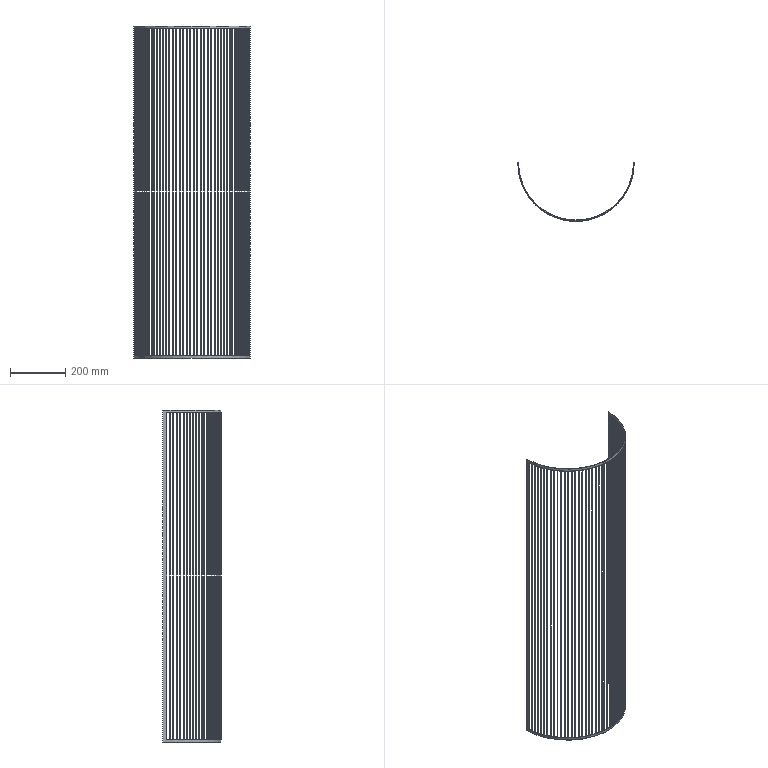Part | SolidWorks | features BaseBody 1 | 1 solid | 202 faces | box 420 x 210 x 1200 mm | volume 419313 mm3 | plane 200 | cylinder 2 | commonest cylinder face diameters 416 x1 420 x1